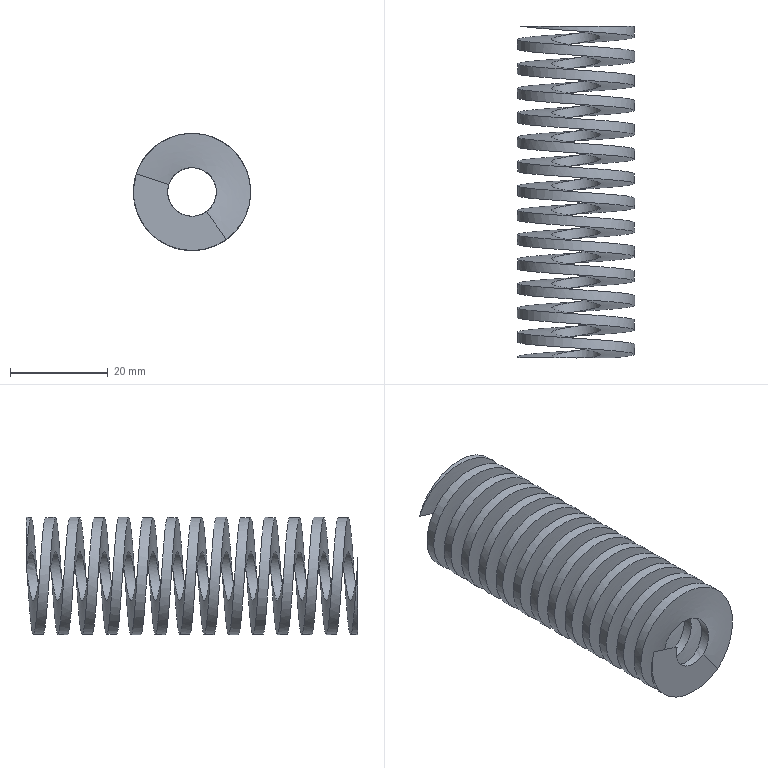Part | STEP file | spring 4_SUS304 | 1 solid | 6 faces | box 24 x 68 x 24 mm | volume 10180 mm3 | spline 4 | plane 2